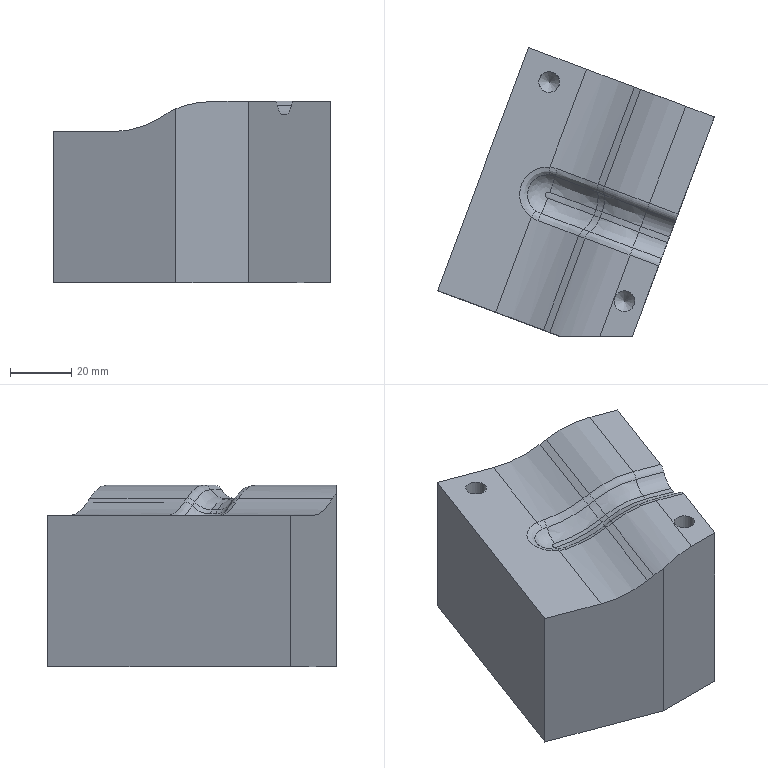Part | NX | features 23 2 | 1 solid | 57 faces | box 90.651 x 94.59 x 59.5 mm | volume 273156 mm3 | cylinder 23 | plane 18 | spline 11 | cone 4 | torus 1 | commonest cylinder face diameters 15 x5 6 x4 13 x4 6.8 x2 10.3 x2 63 x2